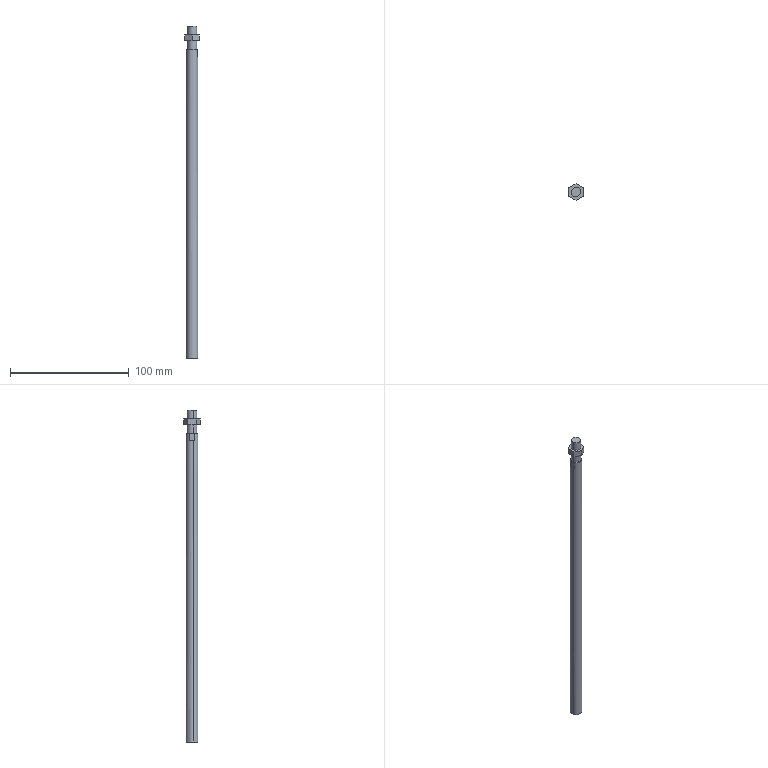Part | SolidWorks | features MBimport 1, MoveFace 1, Scale 1 | 1 solid | 21 faces | box 12 x 13.856 x 280 mm | volume 21775 mm3 | plane 15 | cylinder 6 | commonest cylinder face diameters 8 x4 10 x2
STEP:
#1=CARTESIAN_POINT('',(644.94,-1525.214,-88.08));
#2=VERTEX_POINT('',#1);
#3=CARTESIAN_POINT('',(654.503,-1522.29,-88.08));
#4=VERTEX_POINT('',#3);
#5=CARTESIAN_POINT('',(649.722,-1523.752,-88.08));
#6=DIRECTION('',(0.,0.,1.));
#7=DIRECTION('',(-1.,0.,0.));
#8=AXIS2_PLACEMENT_3D('',#5,#6,#7);
#9=CIRCLE('',#8,5.);
#10=EDGE_CURVE('',#2,#4,#9,.T.);
#11=ORIENTED_EDGE('',*,*,#10,.T.);
#12=CARTESIAN_POINT('',(654.503,-1522.29,165.92));
#13=VERTEX_POINT('',#12);
#14=CARTESIAN_POINT('',(654.503,-1522.29,163.92));
#15=DIRECTION('',(0.,0.,1.));
#16=VECTOR('',#15,1000.);
#17=LINE('',#14,#16);
#18=EDGE_CURVE('',#4,#13,#17,.T.);
#19=ORIENTED_EDGE('',*,*,#18,.T.);
#20=CARTESIAN_POINT('',(654.122,-1526.127,165.92));
#21=VERTEX_POINT('',#20);
#22=CARTESIAN_POINT('',(649.722,-1523.752,165.92));
#23=DIRECTION('',(0.,0.,-1.));
#24=DIRECTION('',(0.9563,0.2924,0.));
#25=AXIS2_PLACEMENT_3D('',#22,#23,#24);
#26=CIRCLE('',#25,5.);
#27=EDGE_CURVE('',#13,#21,#26,.T.);
#28=ORIENTED_EDGE('',*,*,#27,.T.);
#29=CARTESIAN_POINT('',(654.122,-1526.127,171.92));
#30=VERTEX_POINT('',#29);
#31=CARTESIAN_POINT('',(654.122,-1526.127,168.92));
#32=DIRECTION('',(0.,0.,1.));
#33=VECTOR('',#32,1000.);
#34=LINE('',#31,#33);
#35=EDGE_CURVE('',#21,#30,#34,.T.);
#36=ORIENTED_EDGE('',*,*,#35,.T.);
#37=CARTESIAN_POINT('',(645.322,-1526.127,171.92));
#38=VERTEX_POINT('',#37);
#39=CARTESIAN_POINT('',(649.722,-1523.752,171.92));
#40=DIRECTION('',(0.,0.,-1.));
#41=DIRECTION('',(0.9563,0.2924,0.));
#42=AXIS2_PLACEMENT_3D('',#39,#40,#41);
#43=CIRCLE('',#42,5.);
#44=EDGE_CURVE('',#30,#38,#43,.T.);
#45=ORIENTED_EDGE('',*,*,#44,.T.);
#46=CARTESIAN_POINT('',(645.322,-1526.127,165.92));
#47=VERTEX_POINT('',#46);
#48=CARTESIAN_POINT('',(645.322,-1526.127,168.92));
#49=DIRECTION('',(0.,0.,-1.));
#50=VECTOR('',#49,1000.);
#51=LINE('',#48,#50);
#52=EDGE_CURVE('',#38,#47,#51,.T.);
#53=ORIENTED_EDGE('',*,*,#52,.T.);
#54=CARTESIAN_POINT('',(644.94,-1525.214,165.92));
#55=VERTEX_POINT('',#54);
#56=CARTESIAN_POINT('',(649.722,-1523.752,165.92));
#57=DIRECTION('',(0.,0.,-1.));
#58=DIRECTION('',(0.9563,0.2924,0.));
#59=AXIS2_PLACEMENT_3D('',#56,#57,#58);
#60=CIRCLE('',#59,5.);
#61=EDGE_CURVE('',#47,#55,#60,.T.);
#62=ORIENTED_EDGE('',*,*,#61,.T.);
#63=CARTESIAN_POINT('',(644.94,-1525.214,163.92));
#64=DIRECTION('',(0.,0.,1.));
#65=VECTOR('',#64,1000.);
#66=LINE('',#63,#65);
#67=EDGE_CURVE('',#2,#55,#66,.T.);
#68=ORIENTED_EDGE('',*,*,#67,.F.);
#69=EDGE_LOOP('',(#11,#19,#28,#36,#45,#53,#62,#68));
#70=FACE_OUTER_BOUND('',#69,.T.);
#71=CARTESIAN_POINT('',(649.722,-1523.752,163.92));
#72=DIRECTION('',(0.,0.,1.));
#73=DIRECTION('',(-0.9563,-0.2924,0.));
#74=AXIS2_PLACEMENT_3D('',#71,#72,#73);
#75=CYLINDRICAL_SURFACE('',#74,5.);
#76=ADVANCED_FACE('',(#70),#75,.T.);
#77=ORIENTED_EDGE('',*,*,#18,.F.);
#78=CARTESIAN_POINT('',(649.722,-1523.752,-88.08));
#79=DIRECTION('',(0.,0.,1.));
#80=DIRECTION('',(-1.,0.,0.));
#81=AXIS2_PLACEMENT_3D('',#78,#79,#80);
#82=CIRCLE('',#81,5.);
#83=EDGE_CURVE('',#4,#2,#82,.T.);
#84=ORIENTED_EDGE('',*,*,#83,.T.);
#85=ORIENTED_EDGE('',*,*,#67,.T.);
#86=CARTESIAN_POINT('',(645.322,-1521.377,165.92));
#87=VERTEX_POINT('',#86);
#88=CARTESIAN_POINT('',(649.722,-1523.752,165.92));
#89=DIRECTION('',(0.,0.,-1.));
#90=DIRECTION('',(0.9563,0.2924,0.));
#91=AXIS2_PLACEMENT_3D('',#88,#89,#90);
#92=CIRCLE('',#91,5.);
#93=EDGE_CURVE('',#55,#87,#92,.T.);
#94=ORIENTED_EDGE('',*,*,#93,.T.);
#95=CARTESIAN_POINT('',(645.322,-1521.377,171.92));
#96=VERTEX_POINT('',#95);
#97=CARTESIAN_POINT('',(645.322,-1521.377,168.92));
#98=DIRECTION('',(0.,0.,1.));
#99=VECTOR('',#98,1000.);
#100=LINE('',#97,#99);
#101=EDGE_CURVE('',#87,#96,#100,.T.);
#102=ORIENTED_EDGE('',*,*,#101,.T.);
#103=CARTESIAN_POINT('',(654.122,-1521.377,171.92));
#104=VERTEX_POINT('',#103);
#105=CARTESIAN_POINT('',(649.722,-1523.752,171.92));
#106=DIRECTION('',(0.,0.,-1.));
#107=DIRECTION('',(0.9563,0.2924,0.));
#108=AXIS2_PLACEMENT_3D('',#105,#106,#107);
#109=CIRCLE('',#108,5.);
#110=EDGE_CURVE('',#96,#104,#109,.T.);
#111=ORIENTED_EDGE('',*,*,#110,.T.);
#112=CARTESIAN_POINT('',(654.122,-1521.377,165.92));
#113=VERTEX_POINT('',#112);
#114=CARTESIAN_POINT('',(654.122,-1521.377,168.92));
#115=DIRECTION('',(0.,0.,-1.));
#116=VECTOR('',#115,1000.);
#117=LINE('',#114,#116);
#118=EDGE_CURVE('',#104,#113,#117,.T.);
#119=ORIENTED_EDGE('',*,*,#118,.T.);
#120=CARTESIAN_POINT('',(649.722,-1523.752,165.92));
#121=DIRECTION('',(0.,0.,-1.));
#122=DIRECTION('',(0.9563,0.2924,0.));
#123=AXIS2_PLACEMENT_3D('',#120,#121,#122);
#124=CIRCLE('',#123,5.);
#125=EDGE_CURVE('',#113,#13,#124,.T.);
#126=ORIENTED_EDGE('',*,*,#125,.T.);
#127=EDGE_LOOP('',(#77,#84,#85,#94,#102,#111,#119,#126));
#128=FACE_OUTER_BOUND('',#127,.T.);
#129=CARTESIAN_POINT('',(649.722,-1523.752,163.92));
#130=DIRECTION('',(0.,0.,1.));
#131=DIRECTION('',(-0.9563,-0.2924,0.));
#132=AXIS2_PLACEMENT_3D('',#129,#130,#131);
#133=CYLINDRICAL_SURFACE('',#132,5.);
#134=ADVANCED_FACE('',(#128),#133,.T.);
#135=CARTESIAN_POINT('',(653.547,-1522.582,184.42));
#136=VERTEX_POINT('',#135);
#137=CARTESIAN_POINT('',(653.547,-1522.582,191.92));
#138=VERTEX_POINT('',#137);
#139=CARTESIAN_POINT('',(653.547,-1522.582,191.92));
#140=DIRECTION('',(0.,0.,1.));
#141=VECTOR('',#140,1000.);
#142=LINE('',#139,#141);
#143=EDGE_CURVE('',#136,#138,#142,.T.);
#144=ORIENTED_EDGE('',*,*,#143,.F.);
#145=CARTESIAN_POINT('',(645.896,-1524.921,184.42));
#146=VERTEX_POINT('',#145);
#147=CARTESIAN_POINT('',(649.722,-1523.752,184.42));
#148=DIRECTION('',(0.,0.,1.));
#149=DIRECTION('',(0.9563,0.2924,0.));
#150=AXIS2_PLACEMENT_3D('',#147,#148,#149);
#151=CIRCLE('',#150,4.);
#152=EDGE_CURVE('',#136,#146,#151,.T.);
#153=ORIENTED_EDGE('',*,*,#152,.T.);
#154=CARTESIAN_POINT('',(645.896,-1524.921,191.92));
#155=VERTEX_POINT('',#154);
#156=CARTESIAN_POINT('',(645.896,-1524.921,191.92));
#157=DIRECTION('',(0.,0.,-1.));
#158=VECTOR('',#157,1000.);
#159=LINE('',#156,#158);
#160=EDGE_CURVE('',#155,#146,#159,.T.);
#161=ORIENTED_EDGE('',*,*,#160,.F.);
#162=CARTESIAN_POINT('',(649.722,-1523.752,191.92));
#163=DIRECTION('',(0.,0.,1.));
#164=DIRECTION('',(0.9563,0.2924,0.));
#165=AXIS2_PLACEMENT_3D('',#162,#163,#164);
#166=CIRCLE('',#165,4.);
#167=EDGE_CURVE('',#138,#155,#166,.T.);
#168=ORIENTED_EDGE('',*,*,#167,.F.);
#169=EDGE_LOOP('',(#144,#153,#161,#168));
#170=FACE_OUTER_BOUND('',#169,.T.);
#171=CARTESIAN_POINT('',(649.722,-1523.752,191.92));
#172=DIRECTION('',(0.,0.,-1.));
#173=DIRECTION('',(-0.9563,-0.2924,0.));
#174=AXIS2_PLACEMENT_3D('',#171,#172,#173);
#175=CYLINDRICAL_SURFACE('',#174,4.);
#176=ADVANCED_FACE('',(#170),#175,.T.);
#177=CARTESIAN_POINT('',(653.547,-1522.582,171.92));
#178=VERTEX_POINT('',#177);
#179=CARTESIAN_POINT('',(653.547,-1522.582,179.42));
#180=VERTEX_POINT('',#179);
#181=CARTESIAN_POINT('',(653.547,-1522.582,175.67));
#182=DIRECTION('',(0.,0.,1.));
#183=VECTOR('',#182,1000.);
#184=LINE('',#181,#183);
#185=EDGE_CURVE('',#178,#180,#184,.T.);
#186=ORIENTED_EDGE('',*,*,#185,.F.);
#187=CARTESIAN_POINT('',(645.896,-1524.921,171.92));
#188=VERTEX_POINT('',#187);
#189=CARTESIAN_POINT('',(649.722,-1523.752,171.92));
#190=DIRECTION('',(0.,0.,-1.));
#191=DIRECTION('',(0.9563,0.2924,0.));
#192=AXIS2_PLACEMENT_3D('',#189,#190,#191);
#193=CIRCLE('',#192,4.);
#194=EDGE_CURVE('',#188,#178,#193,.T.);
#195=ORIENTED_EDGE('',*,*,#194,.F.);
#196=CARTESIAN_POINT('',(645.896,-1524.921,179.42));
#197=VERTEX_POINT('',#196);
#198=CARTESIAN_POINT('',(645.896,-1524.921,175.67));
#199=DIRECTION('',(0.,0.,-1.));
#200=VECTOR('',#199,1000.);
#201=LINE('',#198,#200);
#202=EDGE_CURVE('',#197,#188,#201,.T.);
#203=ORIENTED_EDGE('',*,*,#202,.F.);
#204=CARTESIAN_POINT('',(649.722,-1523.752,179.42));
#205=DIRECTION('',(0.,0.,-1.));
#206=DIRECTION('',(0.9563,0.2924,0.));
#207=AXIS2_PLACEMENT_3D('',#204,#205,#206);
#208=CIRCLE('',#207,4.);
#209=EDGE_CURVE('',#197,#180,#208,.T.);
#210=ORIENTED_EDGE('',*,*,#209,.T.);
#211=EDGE_LOOP('',(#186,#195,#203,#210));
#212=FACE_OUTER_BOUND('',#211,.T.);
#213=CARTESIAN_POINT('',(649.722,-1523.752,191.92));
#214=DIRECTION('',(0.,0.,-1.));
#215=DIRECTION('',(-0.9563,-0.2924,0.));
#216=AXIS2_PLACEMENT_3D('',#213,#214,#215);
#217=CYLINDRICAL_SURFACE('',#216,4.);
#218=ADVANCED_FACE('',(#212),#217,.T.);
#219=CARTESIAN_POINT('',(655.722,-1520.288,184.42));
#220=VERTEX_POINT('',#219);
#221=CARTESIAN_POINT('',(655.722,-1527.216,184.42));
#222=VERTEX_POINT('',#221);
#223=CARTESIAN_POINT('',(655.722,-1527.216,184.42));
#224=DIRECTION('',(0.,-1.,0.));
#225=VECTOR('',#224,1000.);
#226=LINE('',#223,#225);
#227=EDGE_CURVE('',#220,#222,#226,.T.);
#228=ORIENTED_EDGE('',*,*,#227,.T.);
#229=CARTESIAN_POINT('',(655.722,-1527.216,179.42));
#230=VERTEX_POINT('',#229);
#231=CARTESIAN_POINT('',(655.722,-1527.216,179.42));
#232=DIRECTION('',(0.,0.,1.));
#233=VECTOR('',#232,1000.);
#234=LINE('',#231,#233);
#235=EDGE_CURVE('',#230,#222,#234,.T.);
#236=ORIENTED_EDGE('',*,*,#235,.F.);
#237=CARTESIAN_POINT('',(655.722,-1520.288,179.42));
#238=VERTEX_POINT('',#237);
#239=CARTESIAN_POINT('',(655.722,-1527.216,179.42));
#240=DIRECTION('',(0.,1.,0.));
#241=VECTOR('',#240,1000.);
#242=LINE('',#239,#241);
#243=EDGE_CURVE('',#230,#238,#242,.T.);
#244=ORIENTED_EDGE('',*,*,#243,.T.);
#245=CARTESIAN_POINT('',(655.722,-1520.288,179.42));
#246=DIRECTION('',(0.,0.,1.));
#247=VECTOR('',#246,1000.);
#248=LINE('',#245,#247);
#249=EDGE_CURVE('',#238,#220,#248,.T.);
#250=ORIENTED_EDGE('',*,*,#249,.T.);
#251=EDGE_LOOP('',(#228,#236,#244,#250));
#252=FACE_OUTER_BOUND('',#251,.T.);
#253=CARTESIAN_POINT('',(655.722,-1523.752,179.42));
#254=DIRECTION('',(1.,0.,0.));
#255=DIRECTION('',(0.,1.,0.));
#256=AXIS2_PLACEMENT_3D('',#253,#254,#255);
#257=PLANE('',#256);
#258=ADVANCED_FACE('',(#252),#257,.T.);
#259=CARTESIAN_POINT('',(649.722,-1516.823,184.42));
#260=VERTEX_POINT('',#259);
#261=CARTESIAN_POINT('',(655.722,-1520.288,184.42));
#262=DIRECTION('',(0.866,-0.5,0.));
#263=VECTOR('',#262,1000.);
#264=LINE('',#261,#263);
#265=EDGE_CURVE('',#260,#220,#264,.T.);
#266=ORIENTED_EDGE('',*,*,#265,.T.);
#267=ORIENTED_EDGE('',*,*,#249,.F.);
#268=CARTESIAN_POINT('',(649.722,-1516.823,179.42));
#269=VERTEX_POINT('',#268);
#270=CARTESIAN_POINT('',(655.722,-1520.288,179.42));
#271=DIRECTION('',(-0.866,0.5,0.));
#272=VECTOR('',#271,1000.);
#273=LINE('',#270,#272);
#274=EDGE_CURVE('',#238,#269,#273,.T.);
#275=ORIENTED_EDGE('',*,*,#274,.T.);
#276=CARTESIAN_POINT('',(649.722,-1516.823,179.42));
#277=DIRECTION('',(0.,0.,1.));
#278=VECTOR('',#277,1000.);
#279=LINE('',#276,#278);
#280=EDGE_CURVE('',#269,#260,#279,.T.);
#281=ORIENTED_EDGE('',*,*,#280,.T.);
#282=EDGE_LOOP('',(#266,#267,#275,#281));
#283=FACE_OUTER_BOUND('',#282,.T.);
#284=CARTESIAN_POINT('',(652.722,-1518.555,179.42));
#285=DIRECTION('',(0.5,0.866,0.));
#286=DIRECTION('',(0.,0.,-1.));
#287=AXIS2_PLACEMENT_3D('',#284,#285,#286);
#288=PLANE('',#287);
#289=ADVANCED_FACE('',(#283),#288,.T.);
#290=CARTESIAN_POINT('',(643.722,-1520.288,184.42));
#291=VERTEX_POINT('',#290);
#292=CARTESIAN_POINT('',(649.722,-1516.823,184.42));
#293=DIRECTION('',(0.866,0.5,0.));
#294=VECTOR('',#293,1000.);
#295=LINE('',#292,#294);
#296=EDGE_CURVE('',#291,#260,#295,.T.);
#297=ORIENTED_EDGE('',*,*,#296,.T.);
#298=ORIENTED_EDGE('',*,*,#280,.F.);
#299=CARTESIAN_POINT('',(643.722,-1520.288,179.42));
#300=VERTEX_POINT('',#299);
#301=CARTESIAN_POINT('',(649.722,-1516.823,179.42));
#302=DIRECTION('',(-0.866,-0.5,0.));
#303=VECTOR('',#302,1000.);
#304=LINE('',#301,#303);
#305=EDGE_CURVE('',#269,#300,#304,.T.);
#306=ORIENTED_EDGE('',*,*,#305,.T.);
#307=CARTESIAN_POINT('',(643.722,-1520.288,179.42));
#308=DIRECTION('',(0.,0.,1.));
#309=VECTOR('',#308,1000.);
#310=LINE('',#307,#309);
#311=EDGE_CURVE('',#300,#291,#310,.T.);
#312=ORIENTED_EDGE('',*,*,#311,.T.);
#313=EDGE_LOOP('',(#297,#298,#306,#312));
#314=FACE_OUTER_BOUND('',#313,.T.);
#315=CARTESIAN_POINT('',(646.722,-1518.555,179.42));
#316=DIRECTION('',(-0.5,0.866,0.));
#317=DIRECTION('',(0.,0.,1.));
#318=AXIS2_PLACEMENT_3D('',#315,#316,#317);
#319=PLANE('',#318);
#320=ADVANCED_FACE('',(#314),#319,.T.);
#321=CARTESIAN_POINT('',(643.722,-1527.216,184.42));
#322=VERTEX_POINT('',#321);
#323=CARTESIAN_POINT('',(643.722,-1520.288,184.42));
#324=DIRECTION('',(0.,1.,0.));
#325=VECTOR('',#324,1000.);
#326=LINE('',#323,#325);
#327=EDGE_CURVE('',#322,#291,#326,.T.);
#328=ORIENTED_EDGE('',*,*,#327,.T.);
#329=ORIENTED_EDGE('',*,*,#311,.F.);
#330=CARTESIAN_POINT('',(643.722,-1527.216,179.42));
#331=VERTEX_POINT('',#330);
#332=CARTESIAN_POINT('',(643.722,-1520.288,179.42));
#333=DIRECTION('',(0.,-1.,0.));
#334=VECTOR('',#333,1000.);
#335=LINE('',#332,#334);
#336=EDGE_CURVE('',#300,#331,#335,.T.);
#337=ORIENTED_EDGE('',*,*,#336,.T.);
#338=CARTESIAN_POINT('',(643.722,-1527.216,179.42));
#339=DIRECTION('',(0.,0.,1.));
#340=VECTOR('',#339,1000.);
#341=LINE('',#338,#340);
#342=EDGE_CURVE('',#331,#322,#341,.T.);
#343=ORIENTED_EDGE('',*,*,#342,.T.);
#344=EDGE_LOOP('',(#328,#329,#337,#343));
#345=FACE_OUTER_BOUND('',#344,.T.);
#346=CARTESIAN_POINT('',(643.722,-1523.752,179.42));
#347=DIRECTION('',(-1.,0.,0.));
#348=DIRECTION('',(0.,0.,1.));
#349=AXIS2_PLACEMENT_3D('',#346,#347,#348);
#350=PLANE('',#349);
#351=ADVANCED_FACE('',(#345),#350,.T.);
#352=CARTESIAN_POINT('',(649.722,-1530.68,184.42));
#353=VERTEX_POINT('',#352);
#354=CARTESIAN_POINT('',(643.722,-1527.216,184.42));
#355=DIRECTION('',(-0.866,0.5,0.));
#356=VECTOR('',#355,1000.);
#357=LINE('',#354,#356);
#358=EDGE_CURVE('',#353,#322,#357,.T.);
#359=ORIENTED_EDGE('',*,*,#358,.T.);
#360=ORIENTED_EDGE('',*,*,#342,.F.);
#361=CARTESIAN_POINT('',(649.722,-1530.68,179.42));
#362=VERTEX_POINT('',#361);
#363=CARTESIAN_POINT('',(643.722,-1527.216,179.42));
#364=DIRECTION('',(0.866,-0.5,0.));
#365=VECTOR('',#364,1000.);
#366=LINE('',#363,#365);
#367=EDGE_CURVE('',#331,#362,#366,.T.);
#368=ORIENTED_EDGE('',*,*,#367,.T.);
#369=CARTESIAN_POINT('',(649.722,-1530.68,179.42));
#370=DIRECTION('',(0.,0.,1.));
#371=VECTOR('',#370,1000.);
#372=LINE('',#369,#371);
#373=EDGE_CURVE('',#362,#353,#372,.T.);
#374=ORIENTED_EDGE('',*,*,#373,.T.);
#375=EDGE_LOOP('',(#359,#360,#368,#374));
#376=FACE_OUTER_BOUND('',#375,.T.);
#377=CARTESIAN_POINT('',(646.722,-1528.948,179.42));
#378=DIRECTION('',(-0.5,-0.866,0.));
#379=DIRECTION('',(-0.866,0.5,0.));
#380=AXIS2_PLACEMENT_3D('',#377,#378,#379);
#381=PLANE('',#380);
#382=ADVANCED_FACE('',(#376),#381,.T.);
#383=CARTESIAN_POINT('',(649.722,-1530.68,184.42));
#384=DIRECTION('',(-0.866,-0.5,0.));
#385=VECTOR('',#384,1000.);
#386=LINE('',#383,#385);
#387=EDGE_CURVE('',#222,#353,#386,.T.);
#388=ORIENTED_EDGE('',*,*,#387,.T.);
#389=ORIENTED_EDGE('',*,*,#373,.F.);
#390=CARTESIAN_POINT('',(649.722,-1530.68,179.42));
#391=DIRECTION('',(0.866,0.5,0.));
#392=VECTOR('',#391,1000.);
#393=LINE('',#390,#392);
#394=EDGE_CURVE('',#362,#230,#393,.T.);
#395=ORIENTED_EDGE('',*,*,#394,.T.);
#396=ORIENTED_EDGE('',*,*,#235,.T.);
#397=EDGE_LOOP('',(#388,#389,#395,#396));
#398=FACE_OUTER_BOUND('',#397,.T.);
#399=CARTESIAN_POINT('',(652.722,-1528.948,179.42));
#400=DIRECTION('',(0.5,-0.866,0.));
#401=DIRECTION('',(0.,0.,-1.));
#402=AXIS2_PLACEMENT_3D('',#399,#400,#401);
#403=PLANE('',#402);
#404=ADVANCED_FACE('',(#398),#403,.T.);
#405=ORIENTED_EDGE('',*,*,#227,.F.);
#406=ORIENTED_EDGE('',*,*,#265,.F.);
#407=ORIENTED_EDGE('',*,*,#296,.F.);
#408=ORIENTED_EDGE('',*,*,#327,.F.);
#409=ORIENTED_EDGE('',*,*,#358,.F.);
#410=ORIENTED_EDGE('',*,*,#387,.F.);
#411=EDGE_LOOP('',(#405,#406,#407,#408,#409,#410));
#412=FACE_OUTER_BOUND('',#411,.T.);
#413=CARTESIAN_POINT('',(649.722,-1523.752,184.42));
#414=DIRECTION('',(0.,0.,1.));
#415=DIRECTION('',(0.9563,0.2924,0.));
#416=AXIS2_PLACEMENT_3D('',#413,#414,#415);
#417=CIRCLE('',#416,4.);
#418=EDGE_CURVE('',#146,#136,#417,.T.);
#419=ORIENTED_EDGE('',*,*,#418,.F.);
#420=ORIENTED_EDGE('',*,*,#152,.F.);
#421=EDGE_LOOP('',(#419,#420));
#422=FACE_BOUND('',#421,.T.);
#423=CARTESIAN_POINT('',(649.722,-1523.752,184.42));
#424=DIRECTION('',(0.,0.,1.));
#425=DIRECTION('',(1.,0.,0.));
#426=AXIS2_PLACEMENT_3D('',#423,#424,#425);
#427=PLANE('',#426);
#428=ADVANCED_FACE('',(#412,#422),#427,.T.);
#429=ORIENTED_EDGE('',*,*,#274,.F.);
#430=ORIENTED_EDGE('',*,*,#243,.F.);
#431=ORIENTED_EDGE('',*,*,#394,.F.);
#432=ORIENTED_EDGE('',*,*,#367,.F.);
#433=ORIENTED_EDGE('',*,*,#336,.F.);
#434=ORIENTED_EDGE('',*,*,#305,.F.);
#435=EDGE_LOOP('',(#429,#430,#431,#432,#433,#434));
#436=FACE_OUTER_BOUND('',#435,.T.);
#437=ORIENTED_EDGE('',*,*,#209,.F.);
#438=CARTESIAN_POINT('',(649.722,-1523.752,179.42));
#439=DIRECTION('',(0.,0.,-1.));
#440=DIRECTION('',(0.9563,0.2924,0.));
#441=AXIS2_PLACEMENT_3D('',#438,#439,#440);
#442=CIRCLE('',#441,4.);
#443=EDGE_CURVE('',#180,#197,#442,.T.);
#444=ORIENTED_EDGE('',*,*,#443,.F.);
#445=EDGE_LOOP('',(#437,#444));
#446=FACE_BOUND('',#445,.T.);
#447=CARTESIAN_POINT('',(649.722,-1523.752,179.42));
#448=DIRECTION('',(0.,0.,1.));
#449=DIRECTION('',(1.,0.,0.));
#450=AXIS2_PLACEMENT_3D('',#447,#448,#449);
#451=PLANE('',#450);
#452=ADVANCED_FACE('',(#436,#446),#451,.F.);
#453=ORIENTED_EDGE('',*,*,#185,.T.);
#454=ORIENTED_EDGE('',*,*,#443,.T.);
#455=ORIENTED_EDGE('',*,*,#202,.T.);
#456=CARTESIAN_POINT('',(649.722,-1523.752,171.92));
#457=DIRECTION('',(0.,0.,-1.));
#458=DIRECTION('',(0.9563,0.2924,0.));
#459=AXIS2_PLACEMENT_3D('',#456,#457,#458);
#460=CIRCLE('',#459,4.);
#461=EDGE_CURVE('',#178,#188,#460,.T.);
#462=ORIENTED_EDGE('',*,*,#461,.F.);
#463=EDGE_LOOP('',(#453,#454,#455,#462));
#464=FACE_OUTER_BOUND('',#463,.T.);
#465=CARTESIAN_POINT('',(649.722,-1523.752,191.92));
#466=DIRECTION('',(0.,0.,-1.));
#467=DIRECTION('',(-0.9563,-0.2924,0.));
#468=AXIS2_PLACEMENT_3D('',#465,#466,#467);
#469=CYLINDRICAL_SURFACE('',#468,4.);
#470=ADVANCED_FACE('',(#464),#469,.T.);
#471=ORIENTED_EDGE('',*,*,#125,.F.);
#472=CARTESIAN_POINT('',(654.122,-1521.377,165.92));
#473=DIRECTION('',(0.,-1.,0.));
#474=VECTOR('',#473,1000.);
#475=LINE('',#472,#474);
#476=EDGE_CURVE('',#113,#21,#475,.T.);
#477=ORIENTED_EDGE('',*,*,#476,.T.);
#478=ORIENTED_EDGE('',*,*,#27,.F.);
#479=EDGE_LOOP('',(#471,#477,#478));
#480=FACE_OUTER_BOUND('',#479,.T.);
#481=CARTESIAN_POINT('',(654.305,-1523.752,165.92));
#482=DIRECTION('',(0.,0.,1.));
#483=DIRECTION('',(1.,0.,0.));
#484=AXIS2_PLACEMENT_3D('',#481,#482,#483);
#485=PLANE('',#484);
#486=ADVANCED_FACE('',(#480),#485,.T.);
#487=ORIENTED_EDGE('',*,*,#476,.F.);
#488=ORIENTED_EDGE('',*,*,#118,.F.);
#489=CARTESIAN_POINT('',(654.122,-1523.752,171.92));
#490=DIRECTION('',(0.,1.,0.));
#491=VECTOR('',#490,1000.);
#492=LINE('',#489,#491);
#493=EDGE_CURVE('',#30,#104,#492,.T.);
#494=ORIENTED_EDGE('',*,*,#493,.F.);
#495=ORIENTED_EDGE('',*,*,#35,.F.);
#496=EDGE_LOOP('',(#487,#488,#494,#495));
#497=FACE_OUTER_BOUND('',#496,.T.);
#498=CARTESIAN_POINT('',(654.122,-1523.752,171.92));
#499=DIRECTION('',(-1.,0.,0.));
#500=DIRECTION('',(0.,0.,1.));
#501=AXIS2_PLACEMENT_3D('',#498,#499,#500);
#502=PLANE('',#501);
#503=ADVANCED_FACE('',(#497),#502,.F.);
#504=ORIENTED_EDGE('',*,*,#61,.F.);
#505=CARTESIAN_POINT('',(645.322,-1521.377,165.92));
#506=DIRECTION('',(0.,1.,0.));
#507=VECTOR('',#506,1000.);
#508=LINE('',#505,#507);
#509=EDGE_CURVE('',#47,#87,#508,.T.);
#510=ORIENTED_EDGE('',*,*,#509,.T.);
#511=ORIENTED_EDGE('',*,*,#93,.F.);
#512=EDGE_LOOP('',(#504,#510,#511));
#513=FACE_OUTER_BOUND('',#512,.T.);
#514=CARTESIAN_POINT('',(645.139,-1523.752,165.92));
#515=DIRECTION('',(0.,0.,1.));
#516=DIRECTION('',(1.,0.,0.));
#517=AXIS2_PLACEMENT_3D('',#514,#515,#516);
#518=PLANE('',#517);
#519=ADVANCED_FACE('',(#513),#518,.T.);
#520=ORIENTED_EDGE('',*,*,#509,.F.);
#521=ORIENTED_EDGE('',*,*,#52,.F.);
#522=CARTESIAN_POINT('',(645.322,-1523.752,171.92));
#523=DIRECTION('',(0.,-1.,0.));
#524=VECTOR('',#523,1000.);
#525=LINE('',#522,#524);
#526=EDGE_CURVE('',#96,#38,#525,.T.);
#527=ORIENTED_EDGE('',*,*,#526,.F.);
#528=ORIENTED_EDGE('',*,*,#101,.F.);
#529=EDGE_LOOP('',(#520,#521,#527,#528));
#530=FACE_OUTER_BOUND('',#529,.T.);
#531=CARTESIAN_POINT('',(645.322,-1523.752,171.92));
#532=DIRECTION('',(1.,0.,0.));
#533=DIRECTION('',(0.,1.,0.));
#534=AXIS2_PLACEMENT_3D('',#531,#532,#533);
#535=PLANE('',#534);
#536=ADVANCED_FACE('',(#530),#535,.F.);
#537=ORIENTED_EDGE('',*,*,#493,.T.);
#538=ORIENTED_EDGE('',*,*,#110,.F.);
#539=ORIENTED_EDGE('',*,*,#526,.T.);
#540=ORIENTED_EDGE('',*,*,#44,.F.);
#541=EDGE_LOOP('',(#537,#538,#539,#540));
#542=FACE_OUTER_BOUND('',#541,.T.);
#543=ORIENTED_EDGE('',*,*,#461,.T.);
#544=ORIENTED_EDGE('',*,*,#194,.T.);
#545=EDGE_LOOP('',(#543,#544));
#546=FACE_BOUND('',#545,.T.);
#547=CARTESIAN_POINT('',(649.722,-1523.752,171.92));
#548=DIRECTION('',(0.,0.,1.));
#549=DIRECTION('',(1.,0.,0.));
#550=AXIS2_PLACEMENT_3D('',#547,#548,#549);
#551=PLANE('',#550);
#552=ADVANCED_FACE('',(#542,#546),#551,.T.);
#553=ORIENTED_EDGE('',*,*,#143,.T.);
#554=CARTESIAN_POINT('',(649.722,-1523.752,191.92));
#555=DIRECTION('',(0.,0.,1.));
#556=DIRECTION('',(0.9563,0.2924,0.));
#557=AXIS2_PLACEMENT_3D('',#554,#555,#556);
#558=CIRCLE('',#557,4.);
#559=EDGE_CURVE('',#155,#138,#558,.T.);
#560=ORIENTED_EDGE('',*,*,#559,.F.);
#561=ORIENTED_EDGE('',*,*,#160,.T.);
#562=ORIENTED_EDGE('',*,*,#418,.T.);
#563=EDGE_LOOP('',(#553,#560,#561,#562));
#564=FACE_OUTER_BOUND('',#563,.T.);
#565=CARTESIAN_POINT('',(649.722,-1523.752,191.92));
#566=DIRECTION('',(0.,0.,-1.));
#567=DIRECTION('',(-0.9563,-0.2924,0.));
#568=AXIS2_PLACEMENT_3D('',#565,#566,#567);
#569=CYLINDRICAL_SURFACE('',#568,4.);
#570=ADVANCED_FACE('',(#564),#569,.T.);
#571=ORIENTED_EDGE('',*,*,#167,.T.);
#572=ORIENTED_EDGE('',*,*,#559,.T.);
#573=EDGE_LOOP('',(#571,#572));
#574=FACE_OUTER_BOUND('',#573,.T.);
#575=CARTESIAN_POINT('',(649.722,-1523.752,191.92));
#576=DIRECTION('',(0.,0.,1.));
#577=DIRECTION('',(1.,0.,0.));
#578=AXIS2_PLACEMENT_3D('',#575,#576,#577);
#579=PLANE('',#578);
#580=ADVANCED_FACE('',(#574),#579,.T.);
#581=ORIENTED_EDGE('',*,*,#10,.F.);
#582=ORIENTED_EDGE('',*,*,#83,.F.);
#583=EDGE_LOOP('',(#581,#582));
#584=FACE_OUTER_BOUND('',#583,.T.);
#585=CARTESIAN_POINT('',(649.722,-1523.752,-88.08));
#586=DIRECTION('',(0.,0.,-1.));
#587=DIRECTION('',(0.,-1.,0.));
#588=AXIS2_PLACEMENT_3D('',#585,#586,#587);
#589=PLANE('',#588);
#590=ADVANCED_FACE('',(#584),#589,.T.);
#591=CLOSED_SHELL('',(#76,#134,#176,#218,#258,#289,#320,#351,#382,#404,#428,#452,#470,#486,#503,#519,#536,#552,#570,#580,#590));
#592=MANIFOLD_SOLID_BREP('',#591);
#593=CARTESIAN_POINT('',(0.,0.,0.));
#594=DIRECTION('',(0.,0.,1.));
#595=DIRECTION('',(1.,0.,0.));
#596=AXIS2_PLACEMENT_3D('',#593,#594,#595);
#597=(LENGTH_UNIT()NAMED_UNIT(*)SI_UNIT(.MILLI.,.METRE.));
#598=UNCERTAINTY_MEASURE_WITH_UNIT(LENGTH_MEASURE(0.00001),#597,'','');
#599=(NAMED_UNIT(*)PLANE_ANGLE_UNIT()SI_UNIT($,.RADIAN.));
#600=(NAMED_UNIT(*)SI_UNIT($,.STERADIAN.)SOLID_ANGLE_UNIT());
#601=(GEOMETRIC_REPRESENTATION_CONTEXT(3)GLOBAL_UNCERTAINTY_ASSIGNED_CONTEXT((#598))GLOBAL_UNIT_ASSIGNED_CONTEXT((#597,#599,#600))REPRESENTATION_CONTEXT('',''));
#602=ADVANCED_BREP_SHAPE_REPRESENTATION('',(#592,#596),#601);